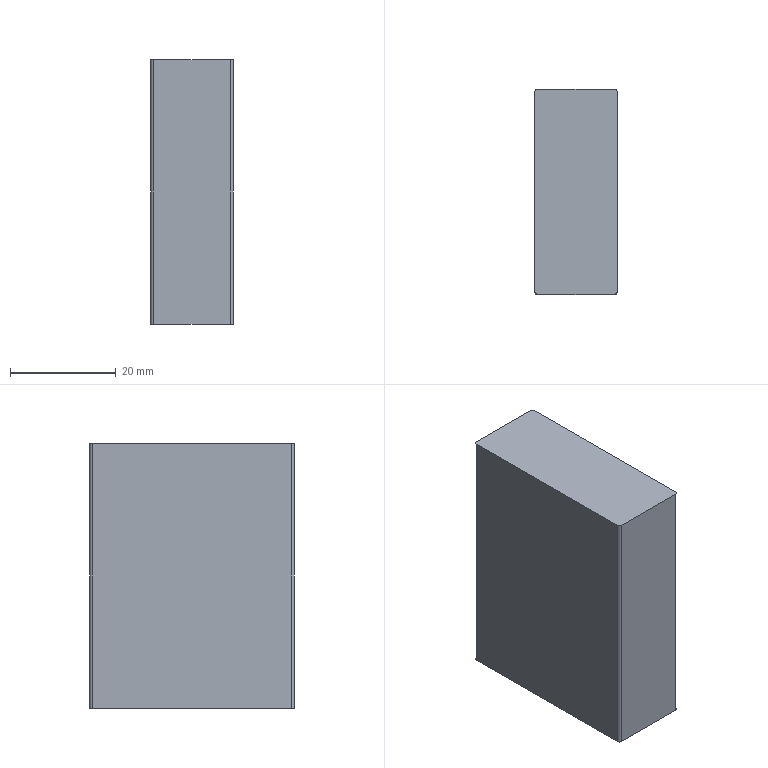Part | NX | features BREP 1 | 1 solid | 10 faces | box 15.542 x 38.72 x 50 mm | volume 30078 mm3 | plane 6 | cylinder 4 | commonest cylinder face diameters 1 x4
STEP:
#1=CARTESIAN_POINT('',(-7.271,19.36,-40.6));
#2=VERTEX_POINT('',#1);
#3=CARTESIAN_POINT('',(-7.771,18.86,-40.6));
#4=VERTEX_POINT('',#3);
#5=CARTESIAN_POINT('',(-7.271,18.86,-40.6));
#6=DIRECTION('',(0.,0.,1.));
#7=DIRECTION('',(1.,0.,0.));
#8=AXIS2_PLACEMENT_3D('',#5,#6,#7);
#9=CIRCLE('',#8,0.5);
#10=EDGE_CURVE('',#2,#4,#9,.T.);
#11=ORIENTED_EDGE('',*,*,#10,.F.);
#12=CARTESIAN_POINT('',(-7.271,19.36,-90.6));
#13=VERTEX_POINT('',#12);
#14=CARTESIAN_POINT('',(-7.271,19.36,-90.6));
#15=DIRECTION('',(0.,0.,1.));
#16=VECTOR('',#15,1000.);
#17=LINE('',#14,#16);
#18=EDGE_CURVE('',#13,#2,#17,.T.);
#19=ORIENTED_EDGE('',*,*,#18,.F.);
#20=CARTESIAN_POINT('',(-7.771,18.86,-90.6));
#21=VERTEX_POINT('',#20);
#22=CARTESIAN_POINT('',(-7.271,18.86,-90.6));
#23=DIRECTION('',(0.,0.,1.));
#24=DIRECTION('',(1.,0.,0.));
#25=AXIS2_PLACEMENT_3D('',#22,#23,#24);
#26=CIRCLE('',#25,0.5);
#27=EDGE_CURVE('',#13,#21,#26,.T.);
#28=ORIENTED_EDGE('',*,*,#27,.T.);
#29=CARTESIAN_POINT('',(-7.771,18.86,-90.6));
#30=DIRECTION('',(0.,0.,1.));
#31=VECTOR('',#30,1000.);
#32=LINE('',#29,#31);
#33=EDGE_CURVE('',#21,#4,#32,.T.);
#34=ORIENTED_EDGE('',*,*,#33,.T.);
#35=EDGE_LOOP('',(#11,#19,#28,#34));
#36=FACE_BOUND('',#35,.T.);
#37=CARTESIAN_POINT('',(-7.271,18.86,-90.6));
#38=DIRECTION('',(0.,0.,1.));
#39=DIRECTION('',(-1.,0.,0.));
#40=AXIS2_PLACEMENT_3D('',#37,#38,#39);
#41=CYLINDRICAL_SURFACE('',#40,0.5);
#42=ADVANCED_FACE('',(#36),#41,.T.);
#43=CARTESIAN_POINT('',(-7.771,-18.86,-40.6));
#44=VERTEX_POINT('',#43);
#45=CARTESIAN_POINT('',(-7.771,-18.86,-40.6));
#46=DIRECTION('',(0.,1.,0.));
#47=VECTOR('',#46,1000.);
#48=LINE('',#45,#47);
#49=EDGE_CURVE('',#44,#4,#48,.T.);
#50=ORIENTED_EDGE('',*,*,#49,.T.);
#51=ORIENTED_EDGE('',*,*,#33,.F.);
#52=CARTESIAN_POINT('',(-7.771,-18.86,-90.6));
#53=VERTEX_POINT('',#52);
#54=CARTESIAN_POINT('',(-7.771,-18.86,-90.6));
#55=DIRECTION('',(0.,1.,0.));
#56=VECTOR('',#55,1000.);
#57=LINE('',#54,#56);
#58=EDGE_CURVE('',#53,#21,#57,.T.);
#59=ORIENTED_EDGE('',*,*,#58,.F.);
#60=CARTESIAN_POINT('',(-7.771,-18.86,-90.6));
#61=DIRECTION('',(0.,0.,1.));
#62=VECTOR('',#61,1000.);
#63=LINE('',#60,#62);
#64=EDGE_CURVE('',#53,#44,#63,.T.);
#65=ORIENTED_EDGE('',*,*,#64,.T.);
#66=EDGE_LOOP('',(#50,#51,#59,#65));
#67=FACE_BOUND('',#66,.T.);
#68=CARTESIAN_POINT('',(-7.771,-18.86,-90.6));
#69=DIRECTION('',(1.,0.,0.));
#70=DIRECTION('',(0.,0.,1.));
#71=AXIS2_PLACEMENT_3D('',#68,#69,#70);
#72=PLANE('',#71);
#73=ADVANCED_FACE('',(#67),#72,.F.);
#74=CARTESIAN_POINT('',(-7.271,-19.36,-40.6));
#75=VERTEX_POINT('',#74);
#76=CARTESIAN_POINT('',(-7.271,-18.86,-40.6));
#77=DIRECTION('',(0.,0.,1.));
#78=DIRECTION('',(1.,0.,0.));
#79=AXIS2_PLACEMENT_3D('',#76,#77,#78);
#80=CIRCLE('',#79,0.5);
#81=EDGE_CURVE('',#44,#75,#80,.T.);
#82=ORIENTED_EDGE('',*,*,#81,.F.);
#83=ORIENTED_EDGE('',*,*,#64,.F.);
#84=CARTESIAN_POINT('',(-7.271,-19.36,-90.6));
#85=VERTEX_POINT('',#84);
#86=CARTESIAN_POINT('',(-7.271,-18.86,-90.6));
#87=DIRECTION('',(0.,0.,1.));
#88=DIRECTION('',(1.,0.,0.));
#89=AXIS2_PLACEMENT_3D('',#86,#87,#88);
#90=CIRCLE('',#89,0.5);
#91=EDGE_CURVE('',#53,#85,#90,.T.);
#92=ORIENTED_EDGE('',*,*,#91,.T.);
#93=CARTESIAN_POINT('',(-7.271,-19.36,-90.6));
#94=DIRECTION('',(0.,0.,1.));
#95=VECTOR('',#94,1000.);
#96=LINE('',#93,#95);
#97=EDGE_CURVE('',#85,#75,#96,.T.);
#98=ORIENTED_EDGE('',*,*,#97,.T.);
#99=EDGE_LOOP('',(#82,#83,#92,#98));
#100=FACE_BOUND('',#99,.T.);
#101=CARTESIAN_POINT('',(-7.271,-18.86,-90.6));
#102=DIRECTION('',(0.,0.,1.));
#103=DIRECTION('',(-1.,0.,0.));
#104=AXIS2_PLACEMENT_3D('',#101,#102,#103);
#105=CYLINDRICAL_SURFACE('',#104,0.5);
#106=ADVANCED_FACE('',(#100),#105,.T.);
#107=CARTESIAN_POINT('',(7.271,-19.36,-40.6));
#108=VERTEX_POINT('',#107);
#109=CARTESIAN_POINT('',(7.271,-19.36,-40.6));
#110=DIRECTION('',(-1.,0.,0.));
#111=VECTOR('',#110,1000.);
#112=LINE('',#109,#111);
#113=EDGE_CURVE('',#108,#75,#112,.T.);
#114=ORIENTED_EDGE('',*,*,#113,.T.);
#115=ORIENTED_EDGE('',*,*,#97,.F.);
#116=CARTESIAN_POINT('',(7.271,-19.36,-90.6));
#117=VERTEX_POINT('',#116);
#118=CARTESIAN_POINT('',(7.271,-19.36,-90.6));
#119=DIRECTION('',(-1.,0.,0.));
#120=VECTOR('',#119,1000.);
#121=LINE('',#118,#120);
#122=EDGE_CURVE('',#117,#85,#121,.T.);
#123=ORIENTED_EDGE('',*,*,#122,.F.);
#124=CARTESIAN_POINT('',(7.271,-19.36,-90.6));
#125=DIRECTION('',(0.,0.,1.));
#126=VECTOR('',#125,1000.);
#127=LINE('',#124,#126);
#128=EDGE_CURVE('',#117,#108,#127,.T.);
#129=ORIENTED_EDGE('',*,*,#128,.T.);
#130=EDGE_LOOP('',(#114,#115,#123,#129));
#131=FACE_BOUND('',#130,.T.);
#132=CARTESIAN_POINT('',(7.271,-19.36,-90.6));
#133=DIRECTION('',(0.,1.,0.));
#134=DIRECTION('',(1.,0.,0.));
#135=AXIS2_PLACEMENT_3D('',#132,#133,#134);
#136=PLANE('',#135);
#137=ADVANCED_FACE('',(#131),#136,.F.);
#138=CARTESIAN_POINT('',(7.771,-18.86,-40.6));
#139=VERTEX_POINT('',#138);
#140=CARTESIAN_POINT('',(7.271,-18.86,-40.6));
#141=DIRECTION('',(0.,0.,1.));
#142=DIRECTION('',(1.,0.,0.));
#143=AXIS2_PLACEMENT_3D('',#140,#141,#142);
#144=CIRCLE('',#143,0.5);
#145=EDGE_CURVE('',#108,#139,#144,.T.);
#146=ORIENTED_EDGE('',*,*,#145,.F.);
#147=ORIENTED_EDGE('',*,*,#128,.F.);
#148=CARTESIAN_POINT('',(7.771,-18.86,-90.6));
#149=VERTEX_POINT('',#148);
#150=CARTESIAN_POINT('',(7.271,-18.86,-90.6));
#151=DIRECTION('',(0.,0.,1.));
#152=DIRECTION('',(1.,0.,0.));
#153=AXIS2_PLACEMENT_3D('',#150,#151,#152);
#154=CIRCLE('',#153,0.5);
#155=EDGE_CURVE('',#117,#149,#154,.T.);
#156=ORIENTED_EDGE('',*,*,#155,.T.);
#157=CARTESIAN_POINT('',(7.771,-18.86,-90.6));
#158=DIRECTION('',(0.,0.,1.));
#159=VECTOR('',#158,1000.);
#160=LINE('',#157,#159);
#161=EDGE_CURVE('',#149,#139,#160,.T.);
#162=ORIENTED_EDGE('',*,*,#161,.T.);
#163=EDGE_LOOP('',(#146,#147,#156,#162));
#164=FACE_BOUND('',#163,.T.);
#165=CARTESIAN_POINT('',(7.271,-18.86,-90.6));
#166=DIRECTION('',(0.,0.,1.));
#167=DIRECTION('',(-1.,0.,0.));
#168=AXIS2_PLACEMENT_3D('',#165,#166,#167);
#169=CYLINDRICAL_SURFACE('',#168,0.5);
#170=ADVANCED_FACE('',(#164),#169,.T.);
#171=CARTESIAN_POINT('',(7.771,18.86,-40.6));
#172=VERTEX_POINT('',#171);
#173=CARTESIAN_POINT('',(7.771,18.86,-40.6));
#174=DIRECTION('',(0.,-1.,0.));
#175=VECTOR('',#174,1000.);
#176=LINE('',#173,#175);
#177=EDGE_CURVE('',#172,#139,#176,.T.);
#178=ORIENTED_EDGE('',*,*,#177,.T.);
#179=ORIENTED_EDGE('',*,*,#161,.F.);
#180=CARTESIAN_POINT('',(7.771,18.86,-90.6));
#181=VERTEX_POINT('',#180);
#182=CARTESIAN_POINT('',(7.771,18.86,-90.6));
#183=DIRECTION('',(0.,-1.,0.));
#184=VECTOR('',#183,1000.);
#185=LINE('',#182,#184);
#186=EDGE_CURVE('',#181,#149,#185,.T.);
#187=ORIENTED_EDGE('',*,*,#186,.F.);
#188=CARTESIAN_POINT('',(7.771,18.86,-90.6));
#189=DIRECTION('',(0.,0.,1.));
#190=VECTOR('',#189,1000.);
#191=LINE('',#188,#190);
#192=EDGE_CURVE('',#181,#172,#191,.T.);
#193=ORIENTED_EDGE('',*,*,#192,.T.);
#194=EDGE_LOOP('',(#178,#179,#187,#193));
#195=FACE_BOUND('',#194,.T.);
#196=CARTESIAN_POINT('',(7.771,18.86,-90.6));
#197=DIRECTION('',(-1.,0.,0.));
#198=DIRECTION('',(0.,0.,-1.));
#199=AXIS2_PLACEMENT_3D('',#196,#197,#198);
#200=PLANE('',#199);
#201=ADVANCED_FACE('',(#195),#200,.F.);
#202=CARTESIAN_POINT('',(7.271,19.36,-40.6));
#203=VERTEX_POINT('',#202);
#204=CARTESIAN_POINT('',(7.271,18.86,-40.6));
#205=DIRECTION('',(0.,0.,1.));
#206=DIRECTION('',(1.,0.,0.));
#207=AXIS2_PLACEMENT_3D('',#204,#205,#206);
#208=CIRCLE('',#207,0.5);
#209=EDGE_CURVE('',#172,#203,#208,.T.);
#210=ORIENTED_EDGE('',*,*,#209,.F.);
#211=ORIENTED_EDGE('',*,*,#192,.F.);
#212=CARTESIAN_POINT('',(7.271,19.36,-90.6));
#213=VERTEX_POINT('',#212);
#214=CARTESIAN_POINT('',(7.271,18.86,-90.6));
#215=DIRECTION('',(0.,0.,1.));
#216=DIRECTION('',(1.,0.,0.));
#217=AXIS2_PLACEMENT_3D('',#214,#215,#216);
#218=CIRCLE('',#217,0.5);
#219=EDGE_CURVE('',#181,#213,#218,.T.);
#220=ORIENTED_EDGE('',*,*,#219,.T.);
#221=CARTESIAN_POINT('',(7.271,19.36,-90.6));
#222=DIRECTION('',(0.,0.,1.));
#223=VECTOR('',#222,1000.);
#224=LINE('',#221,#223);
#225=EDGE_CURVE('',#213,#203,#224,.T.);
#226=ORIENTED_EDGE('',*,*,#225,.T.);
#227=EDGE_LOOP('',(#210,#211,#220,#226));
#228=FACE_BOUND('',#227,.T.);
#229=CARTESIAN_POINT('',(7.271,18.86,-90.6));
#230=DIRECTION('',(0.,0.,1.));
#231=DIRECTION('',(-1.,0.,0.));
#232=AXIS2_PLACEMENT_3D('',#229,#230,#231);
#233=CYLINDRICAL_SURFACE('',#232,0.5);
#234=ADVANCED_FACE('',(#228),#233,.T.);
#235=CARTESIAN_POINT('',(-7.271,19.36,-40.6));
#236=DIRECTION('',(1.,0.,0.));
#237=VECTOR('',#236,1000.);
#238=LINE('',#235,#237);
#239=EDGE_CURVE('',#2,#203,#238,.T.);
#240=ORIENTED_EDGE('',*,*,#239,.T.);
#241=ORIENTED_EDGE('',*,*,#225,.F.);
#242=CARTESIAN_POINT('',(-7.271,19.36,-90.6));
#243=DIRECTION('',(1.,0.,0.));
#244=VECTOR('',#243,1000.);
#245=LINE('',#242,#244);
#246=EDGE_CURVE('',#13,#213,#245,.T.);
#247=ORIENTED_EDGE('',*,*,#246,.F.);
#248=ORIENTED_EDGE('',*,*,#18,.T.);
#249=EDGE_LOOP('',(#240,#241,#247,#248));
#250=FACE_BOUND('',#249,.T.);
#251=CARTESIAN_POINT('',(-7.271,19.36,-90.6));
#252=DIRECTION('',(0.,-1.,0.));
#253=DIRECTION('',(-1.,0.,0.));
#254=AXIS2_PLACEMENT_3D('',#251,#252,#253);
#255=PLANE('',#254);
#256=ADVANCED_FACE('',(#250),#255,.F.);
#257=ORIENTED_EDGE('',*,*,#27,.F.);
#258=ORIENTED_EDGE('',*,*,#246,.T.);
#259=ORIENTED_EDGE('',*,*,#219,.F.);
#260=ORIENTED_EDGE('',*,*,#186,.T.);
#261=ORIENTED_EDGE('',*,*,#155,.F.);
#262=ORIENTED_EDGE('',*,*,#122,.T.);
#263=ORIENTED_EDGE('',*,*,#91,.F.);
#264=ORIENTED_EDGE('',*,*,#58,.T.);
#265=EDGE_LOOP('',(#257,#258,#259,#260,#261,#262,#263,#264));
#266=FACE_BOUND('',#265,.T.);
#267=CARTESIAN_POINT('',(-7.271,18.86,-90.6));
#268=DIRECTION('',(0.,0.,1.));
#269=DIRECTION('',(-1.,0.,0.));
#270=AXIS2_PLACEMENT_3D('',#267,#268,#269);
#271=PLANE('',#270);
#272=ADVANCED_FACE('',(#266),#271,.F.);
#273=ORIENTED_EDGE('',*,*,#10,.T.);
#274=ORIENTED_EDGE('',*,*,#49,.F.);
#275=ORIENTED_EDGE('',*,*,#81,.T.);
#276=ORIENTED_EDGE('',*,*,#113,.F.);
#277=ORIENTED_EDGE('',*,*,#145,.T.);
#278=ORIENTED_EDGE('',*,*,#177,.F.);
#279=ORIENTED_EDGE('',*,*,#209,.T.);
#280=ORIENTED_EDGE('',*,*,#239,.F.);
#281=EDGE_LOOP('',(#273,#274,#275,#276,#277,#278,#279,#280));
#282=FACE_BOUND('',#281,.T.);
#283=CARTESIAN_POINT('',(-7.271,18.86,-40.6));
#284=DIRECTION('',(0.,0.,1.));
#285=DIRECTION('',(-1.,0.,0.));
#286=AXIS2_PLACEMENT_3D('',#283,#284,#285);
#287=PLANE('',#286);
#288=ADVANCED_FACE('',(#282),#287,.T.);
#289=CLOSED_SHELL('',(#42,#73,#106,#137,#170,#201,#234,#256,#272,#288));
#290=MANIFOLD_SOLID_BREP('',#289);
#291=(LENGTH_UNIT()NAMED_UNIT(*)SI_UNIT(.MILLI.,.METRE.));
#292=UNCERTAINTY_MEASURE_WITH_UNIT(LENGTH_MEASURE(0.00001),#291,'','');
#293=(NAMED_UNIT(*)PLANE_ANGLE_UNIT()SI_UNIT($,.RADIAN.));
#294=(NAMED_UNIT(*)SI_UNIT($,.STERADIAN.)SOLID_ANGLE_UNIT());
#295=(GEOMETRIC_REPRESENTATION_CONTEXT(3)GLOBAL_UNCERTAINTY_ASSIGNED_CONTEXT((#292))GLOBAL_UNIT_ASSIGNED_CONTEXT((#291,#293,#294))REPRESENTATION_CONTEXT('',''));
#296=ADVANCED_BREP_SHAPE_REPRESENTATION('',(#290),#295);